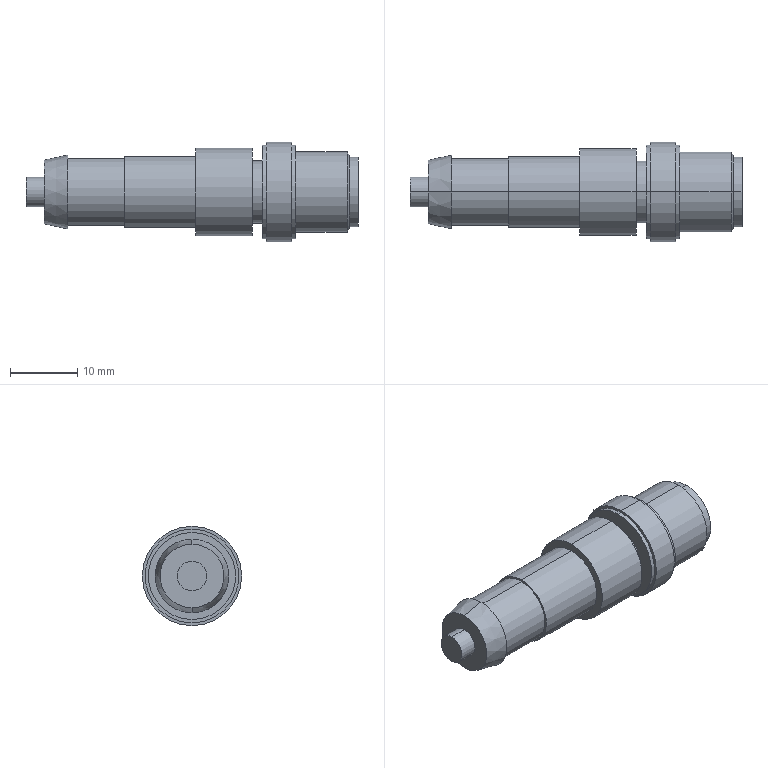Part | STEP file | OP-88071-Part-2-3 | 1 solid | 56 faces | box 49.5 x 14.8 x 14.8 mm | volume 4659 mm3 | cylinder 33 | plane 19 | cone 4 | commonest cylinder face diameters 1 x8 14 x4 8.6 x3 1.2 x2 4.4 x2 9.3 x2
STEP:
#1=CARTESIAN_POINT('',(81.5,2.076,2.924));
#2=VERTEX_POINT('',#1);
#3=CARTESIAN_POINT('',(81.5,2.5,1.9));
#4=VERTEX_POINT('',#3);
#5=CARTESIAN_POINT('',(81.5,2.5,2.5));
#6=DIRECTION('',(1.,0.,0.));
#7=DIRECTION('',(0.,1.,0.));
#8=AXIS2_PLACEMENT_3D('',#5,#6,#7);
#9=CIRCLE('',#8,0.6);
#10=EDGE_CURVE('',#2,#4,#9,.T.);
#11=ORIENTED_EDGE('',*,*,#10,.T.);
#12=CARTESIAN_POINT('',(87.9,2.5,1.9));
#13=VERTEX_POINT('',#12);
#14=CARTESIAN_POINT('',(81.5,2.5,1.9));
#15=DIRECTION('',(1.,0.,0.));
#16=VECTOR('',#15,1000.);
#17=LINE('',#14,#16);
#18=EDGE_CURVE('',#4,#13,#17,.T.);
#19=ORIENTED_EDGE('',*,*,#18,.T.);
#20=CARTESIAN_POINT('',(87.9,2.076,2.924));
#21=VERTEX_POINT('',#20);
#22=CARTESIAN_POINT('',(87.9,2.5,2.5));
#23=DIRECTION('',(1.,0.,0.));
#24=DIRECTION('',(0.,1.,0.));
#25=AXIS2_PLACEMENT_3D('',#22,#23,#24);
#26=CIRCLE('',#25,0.6);
#27=EDGE_CURVE('',#21,#13,#26,.T.);
#28=ORIENTED_EDGE('',*,*,#27,.F.);
#29=CARTESIAN_POINT('',(81.5,2.076,2.924));
#30=DIRECTION('',(1.,0.,0.));
#31=VECTOR('',#30,1000.);
#32=LINE('',#29,#31);
#33=EDGE_CURVE('',#2,#21,#32,.T.);
#34=ORIENTED_EDGE('',*,*,#33,.F.);
#35=EDGE_LOOP('',(#11,#19,#28,#34));
#36=FACE_OUTER_BOUND('',#35,.T.);
#37=CARTESIAN_POINT('',(81.5,2.5,2.5));
#38=DIRECTION('',(1.,0.,0.));
#39=DIRECTION('',(0.,0.,-1.));
#40=AXIS2_PLACEMENT_3D('',#37,#38,#39);
#41=CYLINDRICAL_SURFACE('',#40,0.6);
#42=ADVANCED_FACE('',(#36),#41,.T.);
#43=CARTESIAN_POINT('',(81.5,-2.5,-0.5));
#44=VERTEX_POINT('',#43);
#45=CARTESIAN_POINT('',(81.5,-2.5,0.5));
#46=VERTEX_POINT('',#45);
#47=CARTESIAN_POINT('',(81.5,-2.5,0.));
#48=DIRECTION('',(1.,0.,0.));
#49=DIRECTION('',(0.,1.,0.));
#50=AXIS2_PLACEMENT_3D('',#47,#48,#49);
#51=CIRCLE('',#50,0.5);
#52=EDGE_CURVE('',#44,#46,#51,.T.);
#53=ORIENTED_EDGE('',*,*,#52,.T.);
#54=CARTESIAN_POINT('',(87.9,-2.5,0.5));
#55=VERTEX_POINT('',#54);
#56=CARTESIAN_POINT('',(81.5,-2.5,0.5));
#57=DIRECTION('',(1.,0.,0.));
#58=VECTOR('',#57,1000.);
#59=LINE('',#56,#58);
#60=EDGE_CURVE('',#46,#55,#59,.T.);
#61=ORIENTED_EDGE('',*,*,#60,.T.);
#62=CARTESIAN_POINT('',(87.9,-2.5,-0.5));
#63=VERTEX_POINT('',#62);
#64=CARTESIAN_POINT('',(87.9,-2.5,0.));
#65=DIRECTION('',(1.,0.,0.));
#66=DIRECTION('',(0.,1.,0.));
#67=AXIS2_PLACEMENT_3D('',#64,#65,#66);
#68=CIRCLE('',#67,0.5);
#69=EDGE_CURVE('',#63,#55,#68,.T.);
#70=ORIENTED_EDGE('',*,*,#69,.F.);
#71=CARTESIAN_POINT('',(81.5,-2.5,-0.5));
#72=DIRECTION('',(1.,0.,0.));
#73=VECTOR('',#72,1000.);
#74=LINE('',#71,#73);
#75=EDGE_CURVE('',#44,#63,#74,.T.);
#76=ORIENTED_EDGE('',*,*,#75,.F.);
#77=EDGE_LOOP('',(#53,#61,#70,#76));
#78=FACE_OUTER_BOUND('',#77,.T.);
#79=CARTESIAN_POINT('',(81.5,-2.5,0.));
#80=DIRECTION('',(1.,0.,0.));
#81=DIRECTION('',(0.,0.,-1.));
#82=AXIS2_PLACEMENT_3D('',#79,#80,#81);
#83=CYLINDRICAL_SURFACE('',#82,0.5);
#84=ADVANCED_FACE('',(#78),#83,.T.);
#85=CARTESIAN_POINT('',(81.5,0.,2.));
#86=VERTEX_POINT('',#85);
#87=CARTESIAN_POINT('',(81.5,0.,3.));
#88=VERTEX_POINT('',#87);
#89=CARTESIAN_POINT('',(81.5,0.,2.5));
#90=DIRECTION('',(1.,0.,0.));
#91=DIRECTION('',(0.,1.,0.));
#92=AXIS2_PLACEMENT_3D('',#89,#90,#91);
#93=CIRCLE('',#92,0.5);
#94=EDGE_CURVE('',#86,#88,#93,.T.);
#95=ORIENTED_EDGE('',*,*,#94,.T.);
#96=CARTESIAN_POINT('',(87.9,0.,3.));
#97=VERTEX_POINT('',#96);
#98=CARTESIAN_POINT('',(81.5,0.,3.));
#99=DIRECTION('',(1.,0.,0.));
#100=VECTOR('',#99,1000.);
#101=LINE('',#98,#100);
#102=EDGE_CURVE('',#88,#97,#101,.T.);
#103=ORIENTED_EDGE('',*,*,#102,.T.);
#104=CARTESIAN_POINT('',(87.9,0.,2.));
#105=VERTEX_POINT('',#104);
#106=CARTESIAN_POINT('',(87.9,0.,2.5));
#107=DIRECTION('',(1.,0.,0.));
#108=DIRECTION('',(0.,1.,0.));
#109=AXIS2_PLACEMENT_3D('',#106,#107,#108);
#110=CIRCLE('',#109,0.5);
#111=EDGE_CURVE('',#105,#97,#110,.T.);
#112=ORIENTED_EDGE('',*,*,#111,.F.);
#113=CARTESIAN_POINT('',(81.5,0.,2.));
#114=DIRECTION('',(1.,0.,0.));
#115=VECTOR('',#114,1000.);
#116=LINE('',#113,#115);
#117=EDGE_CURVE('',#86,#105,#116,.T.);
#118=ORIENTED_EDGE('',*,*,#117,.F.);
#119=EDGE_LOOP('',(#95,#103,#112,#118));
#120=FACE_OUTER_BOUND('',#119,.T.);
#121=CARTESIAN_POINT('',(81.5,0.,2.5));
#122=DIRECTION('',(1.,0.,0.));
#123=DIRECTION('',(0.,0.,-1.));
#124=AXIS2_PLACEMENT_3D('',#121,#122,#123);
#125=CYLINDRICAL_SURFACE('',#124,0.5);
#126=ADVANCED_FACE('',(#120),#125,.T.);
#127=CARTESIAN_POINT('',(81.5,0.,-3.));
#128=VERTEX_POINT('',#127);
#129=CARTESIAN_POINT('',(81.5,0.,-2.));
#130=VERTEX_POINT('',#129);
#131=CARTESIAN_POINT('',(81.5,0.,-2.5));
#132=DIRECTION('',(1.,0.,0.));
#133=DIRECTION('',(0.,1.,0.));
#134=AXIS2_PLACEMENT_3D('',#131,#132,#133);
#135=CIRCLE('',#134,0.5);
#136=EDGE_CURVE('',#128,#130,#135,.T.);
#137=ORIENTED_EDGE('',*,*,#136,.T.);
#138=CARTESIAN_POINT('',(87.9,0.,-2.));
#139=VERTEX_POINT('',#138);
#140=CARTESIAN_POINT('',(81.5,0.,-2.));
#141=DIRECTION('',(1.,0.,0.));
#142=VECTOR('',#141,1000.);
#143=LINE('',#140,#142);
#144=EDGE_CURVE('',#130,#139,#143,.T.);
#145=ORIENTED_EDGE('',*,*,#144,.T.);
#146=CARTESIAN_POINT('',(87.9,0.,-3.));
#147=VERTEX_POINT('',#146);
#148=CARTESIAN_POINT('',(87.9,0.,-2.5));
#149=DIRECTION('',(1.,0.,0.));
#150=DIRECTION('',(0.,1.,0.));
#151=AXIS2_PLACEMENT_3D('',#148,#149,#150);
#152=CIRCLE('',#151,0.5);
#153=EDGE_CURVE('',#147,#139,#152,.T.);
#154=ORIENTED_EDGE('',*,*,#153,.F.);
#155=CARTESIAN_POINT('',(81.5,0.,-3.));
#156=DIRECTION('',(1.,0.,0.));
#157=VECTOR('',#156,1000.);
#158=LINE('',#155,#157);
#159=EDGE_CURVE('',#128,#147,#158,.T.);
#160=ORIENTED_EDGE('',*,*,#159,.F.);
#161=EDGE_LOOP('',(#137,#145,#154,#160));
#162=FACE_OUTER_BOUND('',#161,.T.);
#163=CARTESIAN_POINT('',(81.5,0.,-2.5));
#164=DIRECTION('',(1.,0.,0.));
#165=DIRECTION('',(0.,0.,-1.));
#166=AXIS2_PLACEMENT_3D('',#163,#164,#165);
#167=CYLINDRICAL_SURFACE('',#166,0.5);
#168=ADVANCED_FACE('',(#162),#167,.T.);
#169=CARTESIAN_POINT('',(81.5,2.5,-0.5));
#170=VERTEX_POINT('',#169);
#171=CARTESIAN_POINT('',(81.5,2.5,0.5));
#172=VERTEX_POINT('',#171);
#173=CARTESIAN_POINT('',(81.5,2.5,0.));
#174=DIRECTION('',(1.,0.,0.));
#175=DIRECTION('',(0.,1.,0.));
#176=AXIS2_PLACEMENT_3D('',#173,#174,#175);
#177=CIRCLE('',#176,0.5);
#178=EDGE_CURVE('',#170,#172,#177,.T.);
#179=ORIENTED_EDGE('',*,*,#178,.T.);
#180=CARTESIAN_POINT('',(87.9,2.5,0.5));
#181=VERTEX_POINT('',#180);
#182=CARTESIAN_POINT('',(81.5,2.5,0.5));
#183=DIRECTION('',(1.,0.,0.));
#184=VECTOR('',#183,1000.);
#185=LINE('',#182,#184);
#186=EDGE_CURVE('',#172,#181,#185,.T.);
#187=ORIENTED_EDGE('',*,*,#186,.T.);
#188=CARTESIAN_POINT('',(87.9,2.5,-0.5));
#189=VERTEX_POINT('',#188);
#190=CARTESIAN_POINT('',(87.9,2.5,0.));
#191=DIRECTION('',(-1.,0.,0.));
#192=DIRECTION('',(0.,0.,1.));
#193=AXIS2_PLACEMENT_3D('',#190,#191,#192);
#194=CIRCLE('',#193,0.5);
#195=EDGE_CURVE('',#181,#189,#194,.T.);
#196=ORIENTED_EDGE('',*,*,#195,.T.);
#197=CARTESIAN_POINT('',(81.5,2.5,-0.5));
#198=DIRECTION('',(1.,0.,0.));
#199=VECTOR('',#198,1000.);
#200=LINE('',#197,#199);
#201=EDGE_CURVE('',#170,#189,#200,.T.);
#202=ORIENTED_EDGE('',*,*,#201,.F.);
#203=EDGE_LOOP('',(#179,#187,#196,#202));
#204=FACE_OUTER_BOUND('',#203,.T.);
#205=CARTESIAN_POINT('',(81.5,2.5,0.));
#206=DIRECTION('',(1.,0.,0.));
#207=DIRECTION('',(0.,0.,-1.));
#208=AXIS2_PLACEMENT_3D('',#205,#206,#207);
#209=CYLINDRICAL_SURFACE('',#208,0.5);
#210=ADVANCED_FACE('',(#204),#209,.T.);
#211=CARTESIAN_POINT('',(81.5,0.,4.3));
#212=VERTEX_POINT('',#211);
#213=CARTESIAN_POINT('',(81.5,0.,-4.3));
#214=VERTEX_POINT('',#213);
#215=CARTESIAN_POINT('',(81.5,0.,0.));
#216=DIRECTION('',(1.,0.,0.));
#217=DIRECTION('',(0.,1.,0.));
#218=AXIS2_PLACEMENT_3D('',#215,#216,#217);
#219=CIRCLE('',#218,4.3);
#220=EDGE_CURVE('',#212,#214,#219,.T.);
#221=ORIENTED_EDGE('',*,*,#220,.F.);
#222=CARTESIAN_POINT('',(87.9,0.,4.3));
#223=VERTEX_POINT('',#222);
#224=CARTESIAN_POINT('',(81.5,0.,4.3));
#225=DIRECTION('',(1.,0.,0.));
#226=VECTOR('',#225,1000.);
#227=LINE('',#224,#226);
#228=EDGE_CURVE('',#212,#223,#227,.T.);
#229=ORIENTED_EDGE('',*,*,#228,.T.);
#230=CARTESIAN_POINT('',(87.9,0.,-4.3));
#231=VERTEX_POINT('',#230);
#232=CARTESIAN_POINT('',(87.9,0.,0.));
#233=DIRECTION('',(-1.,0.,0.));
#234=DIRECTION('',(0.,0.,1.));
#235=AXIS2_PLACEMENT_3D('',#232,#233,#234);
#236=CIRCLE('',#235,4.3);
#237=EDGE_CURVE('',#231,#223,#236,.T.);
#238=ORIENTED_EDGE('',*,*,#237,.F.);
#239=CARTESIAN_POINT('',(81.5,0.,-4.3));
#240=DIRECTION('',(1.,0.,0.));
#241=VECTOR('',#240,1000.);
#242=LINE('',#239,#241);
#243=EDGE_CURVE('',#214,#231,#242,.T.);
#244=ORIENTED_EDGE('',*,*,#243,.F.);
#245=EDGE_LOOP('',(#221,#229,#238,#244));
#246=FACE_OUTER_BOUND('',#245,.T.);
#247=CARTESIAN_POINT('',(81.5,0.,0.));
#248=DIRECTION('',(1.,0.,0.));
#249=DIRECTION('',(0.,0.,-1.));
#250=AXIS2_PLACEMENT_3D('',#247,#248,#249);
#251=CYLINDRICAL_SURFACE('',#250,4.3);
#252=ADVANCED_FACE('',(#246),#251,.F.);
#253=CARTESIAN_POINT('',(81.5,3.435,2.587));
#254=VERTEX_POINT('',#253);
#255=CARTESIAN_POINT('',(81.5,0.,0.));
#256=DIRECTION('',(1.,0.,0.));
#257=DIRECTION('',(0.,1.,0.));
#258=AXIS2_PLACEMENT_3D('',#255,#256,#257);
#259=CIRCLE('',#258,4.3);
#260=EDGE_CURVE('',#214,#254,#259,.T.);
#261=ORIENTED_EDGE('',*,*,#260,.F.);
#262=ORIENTED_EDGE('',*,*,#243,.T.);
#263=CARTESIAN_POINT('',(87.9,3.435,2.587));
#264=VERTEX_POINT('',#263);
#265=CARTESIAN_POINT('',(87.9,0.,0.));
#266=DIRECTION('',(-1.,0.,0.));
#267=DIRECTION('',(0.,0.,1.));
#268=AXIS2_PLACEMENT_3D('',#265,#266,#267);
#269=CIRCLE('',#268,4.3);
#270=EDGE_CURVE('',#264,#231,#269,.T.);
#271=ORIENTED_EDGE('',*,*,#270,.F.);
#272=CARTESIAN_POINT('',(81.5,3.435,2.587));
#273=DIRECTION('',(1.,0.,0.));
#274=VECTOR('',#273,1000.);
#275=LINE('',#272,#274);
#276=EDGE_CURVE('',#254,#264,#275,.T.);
#277=ORIENTED_EDGE('',*,*,#276,.F.);
#278=EDGE_LOOP('',(#261,#262,#271,#277));
#279=FACE_OUTER_BOUND('',#278,.T.);
#280=CARTESIAN_POINT('',(81.5,0.,0.));
#281=DIRECTION('',(1.,0.,0.));
#282=DIRECTION('',(0.,0.,-1.));
#283=AXIS2_PLACEMENT_3D('',#280,#281,#282);
#284=CYLINDRICAL_SURFACE('',#283,4.3);
#285=ADVANCED_FACE('',(#279),#284,.F.);
#286=CARTESIAN_POINT('',(86.6,0.,-5.2));
#287=VERTEX_POINT('',#286);
#288=CARTESIAN_POINT('',(86.6,0.,5.2));
#289=VERTEX_POINT('',#288);
#290=CARTESIAN_POINT('',(86.6,0.,0.));
#291=DIRECTION('',(1.,0.,0.));
#292=DIRECTION('',(0.,0.,-1.));
#293=AXIS2_PLACEMENT_3D('',#290,#291,#292);
#294=CIRCLE('',#293,5.2);
#295=EDGE_CURVE('',#287,#289,#294,.T.);
#296=ORIENTED_EDGE('',*,*,#295,.T.);
#297=CARTESIAN_POINT('',(87.9,0.,5.2));
#298=VERTEX_POINT('',#297);
#299=CARTESIAN_POINT('',(87.9,0.,5.2));
#300=DIRECTION('',(1.,0.,0.));
#301=VECTOR('',#300,1000.);
#302=LINE('',#299,#301);
#303=EDGE_CURVE('',#289,#298,#302,.T.);
#304=ORIENTED_EDGE('',*,*,#303,.T.);
#305=CARTESIAN_POINT('',(87.9,0.,-5.2));
#306=VERTEX_POINT('',#305);
#307=CARTESIAN_POINT('',(87.9,0.,0.));
#308=DIRECTION('',(1.,0.,0.));
#309=DIRECTION('',(0.,0.,-1.));
#310=AXIS2_PLACEMENT_3D('',#307,#308,#309);
#311=CIRCLE('',#310,5.2);
#312=EDGE_CURVE('',#306,#298,#311,.T.);
#313=ORIENTED_EDGE('',*,*,#312,.F.);
#314=CARTESIAN_POINT('',(87.9,0.,-5.2));
#315=DIRECTION('',(1.,0.,0.));
#316=VECTOR('',#315,1000.);
#317=LINE('',#314,#316);
#318=EDGE_CURVE('',#287,#306,#317,.T.);
#319=ORIENTED_EDGE('',*,*,#318,.F.);
#320=EDGE_LOOP('',(#296,#304,#313,#319));
#321=FACE_OUTER_BOUND('',#320,.T.);
#322=CARTESIAN_POINT('',(87.9,0.,0.));
#323=DIRECTION('',(1.,0.,0.));
#324=DIRECTION('',(0.,0.,-1.));
#325=AXIS2_PLACEMENT_3D('',#322,#323,#324);
#326=CYLINDRICAL_SURFACE('',#325,5.2);
#327=ADVANCED_FACE('',(#321),#326,.T.);
#328=CARTESIAN_POINT('',(86.6,0.,-5.45));
#329=VERTEX_POINT('',#328);
#330=CARTESIAN_POINT('',(86.6,0.,5.45));
#331=VERTEX_POINT('',#330);
#332=CARTESIAN_POINT('',(86.6,0.,0.));
#333=DIRECTION('',(1.,0.,0.));
#334=DIRECTION('',(0.,0.,-1.));
#335=AXIS2_PLACEMENT_3D('',#332,#333,#334);
#336=CIRCLE('',#335,5.45);
#337=EDGE_CURVE('',#329,#331,#336,.T.);
#338=ORIENTED_EDGE('',*,*,#337,.F.);
#339=CARTESIAN_POINT('',(86.3,0.,-6.));
#340=VERTEX_POINT('',#339);
#341=CARTESIAN_POINT('',(86.3,0.,-6.));
#342=DIRECTION('',(-0.4789,0.,-0.8779));
#343=VECTOR('',#342,1000.);
#344=LINE('',#341,#343);
#345=EDGE_CURVE('',#329,#340,#344,.T.);
#346=ORIENTED_EDGE('',*,*,#345,.T.);
#347=CARTESIAN_POINT('',(86.3,0.,6.));
#348=VERTEX_POINT('',#347);
#349=CARTESIAN_POINT('',(86.3,0.,0.));
#350=DIRECTION('',(1.,0.,0.));
#351=DIRECTION('',(0.,0.,-1.));
#352=AXIS2_PLACEMENT_3D('',#349,#350,#351);
#353=CIRCLE('',#352,6.);
#354=EDGE_CURVE('',#340,#348,#353,.T.);
#355=ORIENTED_EDGE('',*,*,#354,.T.);
#356=CARTESIAN_POINT('',(86.3,0.,6.));
#357=DIRECTION('',(-0.4789,0.,0.8779));
#358=VECTOR('',#357,1000.);
#359=LINE('',#356,#358);
#360=EDGE_CURVE('',#331,#348,#359,.T.);
#361=ORIENTED_EDGE('',*,*,#360,.F.);
#362=EDGE_LOOP('',(#338,#346,#355,#361));
#363=FACE_OUTER_BOUND('',#362,.T.);
#364=CARTESIAN_POINT('',(86.3,0.,0.));
#365=DIRECTION('',(-1.,0.,0.));
#366=DIRECTION('',(0.,0.,1.));
#367=AXIS2_PLACEMENT_3D('',#364,#365,#366);
#368=CONICAL_SURFACE('',#367,6.,1.071);
#369=ADVANCED_FACE('',(#363),#368,.T.);
#370=CARTESIAN_POINT('',(78.6,0.,-6.));
#371=VERTEX_POINT('',#370);
#372=CARTESIAN_POINT('',(78.6,0.,6.));
#373=VERTEX_POINT('',#372);
#374=CARTESIAN_POINT('',(78.6,0.,0.));
#375=DIRECTION('',(1.,0.,0.));
#376=DIRECTION('',(0.,0.,-1.));
#377=AXIS2_PLACEMENT_3D('',#374,#375,#376);
#378=CIRCLE('',#377,6.);
#379=EDGE_CURVE('',#371,#373,#378,.T.);
#380=ORIENTED_EDGE('',*,*,#379,.T.);
#381=CARTESIAN_POINT('',(87.9,0.,6.));
#382=DIRECTION('',(1.,0.,0.));
#383=VECTOR('',#382,1000.);
#384=LINE('',#381,#383);
#385=EDGE_CURVE('',#373,#348,#384,.T.);
#386=ORIENTED_EDGE('',*,*,#385,.T.);
#387=ORIENTED_EDGE('',*,*,#354,.F.);
#388=CARTESIAN_POINT('',(87.9,0.,-6.));
#389=DIRECTION('',(1.,0.,0.));
#390=VECTOR('',#389,1000.);
#391=LINE('',#388,#390);
#392=EDGE_CURVE('',#371,#340,#391,.T.);
#393=ORIENTED_EDGE('',*,*,#392,.F.);
#394=EDGE_LOOP('',(#380,#386,#387,#393));
#395=FACE_OUTER_BOUND('',#394,.T.);
#396=CARTESIAN_POINT('',(87.9,0.,0.));
#397=DIRECTION('',(1.,0.,0.));
#398=DIRECTION('',(0.,0.,-1.));
#399=AXIS2_PLACEMENT_3D('',#396,#397,#398);
#400=CYLINDRICAL_SURFACE('',#399,6.);
#401=ADVANCED_FACE('',(#395),#400,.T.);
#402=CARTESIAN_POINT('',(78.,0.,-7.));
#403=VERTEX_POINT('',#402);
#404=CARTESIAN_POINT('',(78.,0.,7.));
#405=VERTEX_POINT('',#404);
#406=CARTESIAN_POINT('',(78.,0.,0.));
#407=DIRECTION('',(1.,0.,0.));
#408=DIRECTION('',(0.,0.,-1.));
#409=AXIS2_PLACEMENT_3D('',#406,#407,#408);
#410=CIRCLE('',#409,7.);
#411=EDGE_CURVE('',#403,#405,#410,.T.);
#412=ORIENTED_EDGE('',*,*,#411,.T.);
#413=CARTESIAN_POINT('',(78.6,0.,7.));
#414=VERTEX_POINT('',#413);
#415=CARTESIAN_POINT('',(87.9,0.,7.));
#416=DIRECTION('',(1.,0.,0.));
#417=VECTOR('',#416,1000.);
#418=LINE('',#415,#417);
#419=EDGE_CURVE('',#405,#414,#418,.T.);
#420=ORIENTED_EDGE('',*,*,#419,.T.);
#421=CARTESIAN_POINT('',(78.6,0.,-7.));
#422=VERTEX_POINT('',#421);
#423=CARTESIAN_POINT('',(78.6,0.,0.));
#424=DIRECTION('',(1.,0.,0.));
#425=DIRECTION('',(0.,0.,-1.));
#426=AXIS2_PLACEMENT_3D('',#423,#424,#425);
#427=CIRCLE('',#426,7.);
#428=EDGE_CURVE('',#422,#414,#427,.T.);
#429=ORIENTED_EDGE('',*,*,#428,.F.);
#430=CARTESIAN_POINT('',(87.9,0.,-7.));
#431=DIRECTION('',(1.,0.,0.));
#432=VECTOR('',#431,1000.);
#433=LINE('',#430,#432);
#434=EDGE_CURVE('',#403,#422,#433,.T.);
#435=ORIENTED_EDGE('',*,*,#434,.F.);
#436=EDGE_LOOP('',(#412,#420,#429,#435));
#437=FACE_OUTER_BOUND('',#436,.T.);
#438=CARTESIAN_POINT('',(87.9,0.,0.));
#439=DIRECTION('',(1.,0.,0.));
#440=DIRECTION('',(0.,0.,-1.));
#441=AXIS2_PLACEMENT_3D('',#438,#439,#440);
#442=CYLINDRICAL_SURFACE('',#441,7.);
#443=ADVANCED_FACE('',(#437),#442,.T.);
#444=CARTESIAN_POINT('',(74.2,0.,-7.4));
#445=VERTEX_POINT('',#444);
#446=CARTESIAN_POINT('',(74.2,0.,7.4));
#447=VERTEX_POINT('',#446);
#448=CARTESIAN_POINT('',(74.2,0.,0.));
#449=DIRECTION('',(1.,0.,0.));
#450=DIRECTION('',(0.,0.,-1.));
#451=AXIS2_PLACEMENT_3D('',#448,#449,#450);
#452=CIRCLE('',#451,7.4);
#453=EDGE_CURVE('',#445,#447,#452,.T.);
#454=ORIENTED_EDGE('',*,*,#453,.T.);
#455=CARTESIAN_POINT('',(78.,0.,7.4));
#456=VERTEX_POINT('',#455);
#457=CARTESIAN_POINT('',(87.9,0.,7.4));
#458=DIRECTION('',(1.,0.,0.));
#459=VECTOR('',#458,1000.);
#460=LINE('',#457,#459);
#461=EDGE_CURVE('',#447,#456,#460,.T.);
#462=ORIENTED_EDGE('',*,*,#461,.T.);
#463=CARTESIAN_POINT('',(78.,0.,-7.4));
#464=VERTEX_POINT('',#463);
#465=CARTESIAN_POINT('',(78.,0.,0.));
#466=DIRECTION('',(1.,0.,0.));
#467=DIRECTION('',(0.,0.,-1.));
#468=AXIS2_PLACEMENT_3D('',#465,#466,#467);
#469=CIRCLE('',#468,7.4);
#470=EDGE_CURVE('',#464,#456,#469,.T.);
#471=ORIENTED_EDGE('',*,*,#470,.F.);
#472=CARTESIAN_POINT('',(87.9,0.,-7.4));
#473=DIRECTION('',(1.,0.,0.));
#474=VECTOR('',#473,1000.);
#475=LINE('',#472,#474);
#476=EDGE_CURVE('',#445,#464,#475,.T.);
#477=ORIENTED_EDGE('',*,*,#476,.F.);
#478=EDGE_LOOP('',(#454,#462,#471,#477));
#479=FACE_OUTER_BOUND('',#478,.T.);
#480=CARTESIAN_POINT('',(87.9,0.,0.));
#481=DIRECTION('',(1.,0.,0.));
#482=DIRECTION('',(0.,0.,-1.));
#483=AXIS2_PLACEMENT_3D('',#480,#481,#482);
#484=CYLINDRICAL_SURFACE('',#483,7.4);
#485=ADVANCED_FACE('',(#479),#484,.T.);
#486=CARTESIAN_POINT('',(73.6,0.,-7.));
#487=VERTEX_POINT('',#486);
#488=CARTESIAN_POINT('',(73.6,0.,7.));
#489=VERTEX_POINT('',#488);
#490=CARTESIAN_POINT('',(73.6,0.,0.));
#491=DIRECTION('',(1.,0.,0.));
#492=DIRECTION('',(0.,0.,-1.));
#493=AXIS2_PLACEMENT_3D('',#490,#491,#492);
#494=CIRCLE('',#493,7.);
#495=EDGE_CURVE('',#487,#489,#494,.T.);
#496=ORIENTED_EDGE('',*,*,#495,.T.);
#497=CARTESIAN_POINT('',(74.2,0.,7.));
#498=VERTEX_POINT('',#497);
#499=CARTESIAN_POINT('',(87.9,0.,7.));
#500=DIRECTION('',(1.,0.,0.));
#501=VECTOR('',#500,1000.);
#502=LINE('',#499,#501);
#503=EDGE_CURVE('',#489,#498,#502,.T.);
#504=ORIENTED_EDGE('',*,*,#503,.T.);
#505=CARTESIAN_POINT('',(74.2,0.,-7.));
#506=VERTEX_POINT('',#505);
#507=CARTESIAN_POINT('',(74.2,0.,0.));
#508=DIRECTION('',(1.,0.,0.));
#509=DIRECTION('',(0.,0.,-1.));
#510=AXIS2_PLACEMENT_3D('',#507,#508,#509);
#511=CIRCLE('',#510,7.);
#512=EDGE_CURVE('',#506,#498,#511,.T.);
#513=ORIENTED_EDGE('',*,*,#512,.F.);
#514=CARTESIAN_POINT('',(87.9,0.,-7.));
#515=DIRECTION('',(1.,0.,0.));
#516=VECTOR('',#515,1000.);
#517=LINE('',#514,#516);
#518=EDGE_CURVE('',#487,#506,#517,.T.);
#519=ORIENTED_EDGE('',*,*,#518,.F.);
#520=EDGE_LOOP('',(#496,#504,#513,#519));
#521=FACE_OUTER_BOUND('',#520,.T.);
#522=CARTESIAN_POINT('',(87.9,0.,0.));
#523=DIRECTION('',(1.,0.,0.));
#524=DIRECTION('',(0.,0.,-1.));
#525=AXIS2_PLACEMENT_3D('',#522,#523,#524);
#526=CYLINDRICAL_SURFACE('',#525,7.);
#527=ADVANCED_FACE('',(#521),#526,.T.);
#528=CARTESIAN_POINT('',(72.1,0.,-4.65));
#529=VERTEX_POINT('',#528);
#530=CARTESIAN_POINT('',(72.1,0.,4.65));
#531=VERTEX_POINT('',#530);
#532=CARTESIAN_POINT('',(72.1,0.,0.));
#533=DIRECTION('',(1.,0.,0.));
#534=DIRECTION('',(0.,0.,-1.));
#535=AXIS2_PLACEMENT_3D('',#532,#533,#534);
#536=CIRCLE('',#535,4.65);
#537=EDGE_CURVE('',#529,#531,#536,.T.);
#538=ORIENTED_EDGE('',*,*,#537,.T.);
#539=CARTESIAN_POINT('',(73.6,0.,4.65));
#540=VERTEX_POINT('',#539);
#541=CARTESIAN_POINT('',(87.9,0.,4.65));
#542=DIRECTION('',(1.,0.,0.));
#543=VECTOR('',#542,1000.);
#544=LINE('',#541,#543);
#545=EDGE_CURVE('',#531,#540,#544,.T.);
#546=ORIENTED_EDGE('',*,*,#545,.T.);
#547=CARTESIAN_POINT('',(73.6,0.,-4.65));
#548=VERTEX_POINT('',#547);
#549=CARTESIAN_POINT('',(73.6,0.,0.));
#550=DIRECTION('',(1.,0.,0.));
#551=DIRECTION('',(0.,0.,-1.));
#552=AXIS2_PLACEMENT_3D('',#549,#550,#551);
#553=CIRCLE('',#552,4.65);
#554=EDGE_CURVE('',#548,#540,#553,.T.);
#555=ORIENTED_EDGE('',*,*,#554,.F.);
#556=CARTESIAN_POINT('',(87.9,0.,-4.65));
#557=DIRECTION('',(1.,0.,0.));
#558=VECTOR('',#557,1000.);
#559=LINE('',#556,#558);
#560=EDGE_CURVE('',#529,#548,#559,.T.);
#561=ORIENTED_EDGE('',*,*,#560,.F.);
#562=EDGE_LOOP('',(#538,#546,#555,#561));
#563=FACE_OUTER_BOUND('',#562,.T.);
#564=CARTESIAN_POINT('',(87.9,0.,0.));
#565=DIRECTION('',(1.,0.,0.));
#566=DIRECTION('',(0.,0.,-1.));
#567=AXIS2_PLACEMENT_3D('',#564,#565,#566);
#568=CYLINDRICAL_SURFACE('',#567,4.65);
#569=ADVANCED_FACE('',(#563),#568,.T.);
#570=CARTESIAN_POINT('',(63.7,0.,-6.5));
#571=VERTEX_POINT('',#570);
#572=CARTESIAN_POINT('',(63.7,0.,6.5));
#573=VERTEX_POINT('',#572);
#574=CARTESIAN_POINT('',(63.7,0.,0.));
#575=DIRECTION('',(1.,0.,0.));
#576=DIRECTION('',(0.,0.,-1.));
#577=AXIS2_PLACEMENT_3D('',#574,#575,#576);
#578=CIRCLE('',#577,6.5);
#579=EDGE_CURVE('',#571,#573,#578,.T.);
#580=ORIENTED_EDGE('',*,*,#579,.T.);
#581=CARTESIAN_POINT('',(72.1,0.,6.5));
#582=VERTEX_POINT('',#581);
#583=CARTESIAN_POINT('',(87.9,0.,6.5));
#584=DIRECTION('',(1.,0.,0.));
#585=VECTOR('',#584,1000.);
#586=LINE('',#583,#585);
#587=EDGE_CURVE('',#573,#582,#586,.T.);
#588=ORIENTED_EDGE('',*,*,#587,.T.);
#589=CARTESIAN_POINT('',(72.1,0.,-6.5));
#590=VERTEX_POINT('',#589);
#591=CARTESIAN_POINT('',(72.1,0.,0.));
#592=DIRECTION('',(1.,0.,0.));
#593=DIRECTION('',(0.,0.,-1.));
#594=AXIS2_PLACEMENT_3D('',#591,#592,#593);
#595=CIRCLE('',#594,6.5);
#596=EDGE_CURVE('',#590,#582,#595,.T.);
#597=ORIENTED_EDGE('',*,*,#596,.F.);
#598=CARTESIAN_POINT('',(87.9,0.,-6.5));
#599=DIRECTION('',(1.,0.,0.));
#600=VECTOR('',#599,1000.);
#601=LINE('',#598,#600);
#602=EDGE_CURVE('',#571,#590,#601,.T.);
#603=ORIENTED_EDGE('',*,*,#602,.F.);
#604=EDGE_LOOP('',(#580,#588,#597,#603));
#605=FACE_OUTER_BOUND('',#604,.T.);
#606=CARTESIAN_POINT('',(87.9,0.,0.));
#607=DIRECTION('',(1.,0.,0.));
#608=DIRECTION('',(0.,0.,-1.));
#609=AXIS2_PLACEMENT_3D('',#606,#607,#608);
#610=CYLINDRICAL_SURFACE('',#609,6.5);
#611=ADVANCED_FACE('',(#605),#610,.T.);
#612=CARTESIAN_POINT('',(53.1,0.,-5.3));
#613=VERTEX_POINT('',#612);
#614=CARTESIAN_POINT('',(53.1,0.,5.3));
#615=VERTEX_POINT('',#614);
#616=CARTESIAN_POINT('',(53.1,0.,0.));
#617=DIRECTION('',(1.,0.,0.));
#618=DIRECTION('',(0.,0.,-1.));
#619=AXIS2_PLACEMENT_3D('',#616,#617,#618);
#620=CIRCLE('',#619,5.3);
#621=EDGE_CURVE('',#613,#615,#620,.T.);
#622=ORIENTED_EDGE('',*,*,#621,.T.);
#623=CARTESIAN_POINT('',(63.7,0.,5.3));
#624=VERTEX_POINT('',#623);
#625=CARTESIAN_POINT('',(87.9,0.,5.3));
#626=DIRECTION('',(1.,0.,0.));
#627=VECTOR('',#626,1000.);
#628=LINE('',#625,#627);
#629=EDGE_CURVE('',#615,#624,#628,.T.);
#630=ORIENTED_EDGE('',*,*,#629,.T.);
#631=CARTESIAN_POINT('',(63.7,0.,-5.3));
#632=VERTEX_POINT('',#631);
#633=CARTESIAN_POINT('',(63.7,0.,0.));
#634=DIRECTION('',(1.,0.,0.));
#635=DIRECTION('',(0.,0.,-1.));
#636=AXIS2_PLACEMENT_3D('',#633,#634,#635);
#637=CIRCLE('',#636,5.3);
#638=EDGE_CURVE('',#632,#624,#637,.T.);
#639=ORIENTED_EDGE('',*,*,#638,.F.);
#640=CARTESIAN_POINT('',(87.9,0.,-5.3));
#641=DIRECTION('',(1.,0.,0.));
#642=VECTOR('',#641,1000.);
#643=LINE('',#640,#642);
#644=EDGE_CURVE('',#613,#632,#643,.T.);
#645=ORIENTED_EDGE('',*,*,#644,.F.);
#646=EDGE_LOOP('',(#622,#630,#639,#645));
#647=FACE_OUTER_BOUND('',#646,.T.);
#648=CARTESIAN_POINT('',(87.9,0.,0.));
#649=DIRECTION('',(1.,0.,0.));
#650=DIRECTION('',(0.,0.,-1.));
#651=AXIS2_PLACEMENT_3D('',#648,#649,#650);
#652=CYLINDRICAL_SURFACE('',#651,5.3);
#653=ADVANCED_FACE('',(#647),#652,.T.);
#654=CARTESIAN_POINT('',(44.6,0.,-5.));
#655=VERTEX_POINT('',#654);
#656=CARTESIAN_POINT('',(44.6,0.,5.));
#657=VERTEX_POINT('',#656);
#658=CARTESIAN_POINT('',(44.6,0.,0.));
#659=DIRECTION('',(1.,0.,0.));
#660=DIRECTION('',(0.,0.,-1.));
#661=AXIS2_PLACEMENT_3D('',#658,#659,#660);
#662=CIRCLE('',#661,5.);
#663=EDGE_CURVE('',#655,#657,#662,.T.);
#664=ORIENTED_EDGE('',*,*,#663,.T.);
#665=CARTESIAN_POINT('',(53.1,0.,5.));
#666=VERTEX_POINT('',#665);
#667=CARTESIAN_POINT('',(87.9,0.,5.));
#668=DIRECTION('',(1.,0.,0.));
#669=VECTOR('',#668,1000.);
#670=LINE('',#667,#669);
#671=EDGE_CURVE('',#657,#666,#670,.T.);
#672=ORIENTED_EDGE('',*,*,#671,.T.);
#673=CARTESIAN_POINT('',(53.1,0.,-5.));
#674=VERTEX_POINT('',#673);
#675=CARTESIAN_POINT('',(53.1,0.,0.));
#676=DIRECTION('',(1.,0.,0.));
#677=DIRECTION('',(0.,0.,-1.));
#678=AXIS2_PLACEMENT_3D('',#675,#676,#677);
#679=CIRCLE('',#678,5.);
#680=EDGE_CURVE('',#674,#666,#679,.T.);
#681=ORIENTED_EDGE('',*,*,#680,.F.);
#682=CARTESIAN_POINT('',(87.9,0.,-5.));
#683=DIRECTION('',(1.,0.,0.));
#684=VECTOR('',#683,1000.);
#685=LINE('',#682,#684);
#686=EDGE_CURVE('',#655,#674,#685,.T.);
#687=ORIENTED_EDGE('',*,*,#686,.F.);
#688=EDGE_LOOP('',(#664,#672,#681,#687));
#689=FACE_OUTER_BOUND('',#688,.T.);
#690=CARTESIAN_POINT('',(87.9,0.,0.));
#691=DIRECTION('',(1.,0.,0.));
#692=DIRECTION('',(0.,0.,-1.));
#693=AXIS2_PLACEMENT_3D('',#690,#691,#692);
#694=CYLINDRICAL_SURFACE('',#693,5.);
#695=ADVANCED_FACE('',(#689),#694,.T.);
#696=CARTESIAN_POINT('',(41.1,0.,-4.75));
#697=VERTEX_POINT('',#696);
#698=CARTESIAN_POINT('',(41.1,0.,4.75));
#699=VERTEX_POINT('',#698);
#700=CARTESIAN_POINT('',(41.1,0.,0.));
#701=DIRECTION('',(1.,0.,0.));
#702=DIRECTION('',(0.,0.,-1.));
#703=AXIS2_PLACEMENT_3D('',#700,#701,#702);
#704=CIRCLE('',#703,4.75);
#705=EDGE_CURVE('',#697,#699,#704,.T.);
#706=ORIENTED_EDGE('',*,*,#705,.T.);
#707=CARTESIAN_POINT('',(44.6,0.,5.5));
#708=VERTEX_POINT('',#707);
#709=CARTESIAN_POINT('',(41.1,0.,4.75));
#710=DIRECTION('',(0.9778,0.,0.2095));
#711=VECTOR('',#710,1000.);
#712=LINE('',#709,#711);
#713=EDGE_CURVE('',#699,#708,#712,.T.);
#714=ORIENTED_EDGE('',*,*,#713,.T.);
#715=CARTESIAN_POINT('',(44.6,0.,-5.5));
#716=VERTEX_POINT('',#715);
#717=CARTESIAN_POINT('',(44.6,0.,0.));
#718=DIRECTION('',(1.,0.,0.));
#719=DIRECTION('',(0.,0.,-1.));
#720=AXIS2_PLACEMENT_3D('',#717,#718,#719);
#721=CIRCLE('',#720,5.5);
#722=EDGE_CURVE('',#716,#708,#721,.T.);
#723=ORIENTED_EDGE('',*,*,#722,.F.);
#724=CARTESIAN_POINT('',(41.1,0.,-4.75));
#725=DIRECTION('',(0.9778,0.,-0.2095));
#726=VECTOR('',#725,1000.);
#727=LINE('',#724,#726);
#728=EDGE_CURVE('',#697,#716,#727,.T.);
#729=ORIENTED_EDGE('',*,*,#728,.F.);
#730=EDGE_LOOP('',(#706,#714,#723,#729));
#731=FACE_OUTER_BOUND('',#730,.T.);
#732=CARTESIAN_POINT('',(41.1,0.,0.));
#733=DIRECTION('',(1.,0.,0.));
#734=DIRECTION('',(0.,0.,-1.));
#735=AXIS2_PLACEMENT_3D('',#732,#733,#734);
#736=CONICAL_SURFACE('',#735,4.75,0.2111);
#737=ADVANCED_FACE('',(#731),#736,.T.);
#738=CARTESIAN_POINT('',(38.4,0.,-2.2));
#739=VERTEX_POINT('',#738);
#740=CARTESIAN_POINT('',(38.4,0.,2.2));
#741=VERTEX_POINT('',#740);
#742=CARTESIAN_POINT('',(38.4,0.,0.));
#743=DIRECTION('',(1.,0.,0.));
#744=DIRECTION('',(0.,0.,-1.));
#745=AXIS2_PLACEMENT_3D('',#742,#743,#744);
#746=CIRCLE('',#745,2.2);
#747=EDGE_CURVE('',#739,#741,#746,.T.);
#748=ORIENTED_EDGE('',*,*,#747,.T.);
#749=CARTESIAN_POINT('',(41.1,0.,2.2));
#750=VERTEX_POINT('',#749);
#751=CARTESIAN_POINT('',(87.9,0.,2.2));
#752=DIRECTION('',(1.,0.,0.));
#753=VECTOR('',#752,1000.);
#754=LINE('',#751,#753);
#755=EDGE_CURVE('',#741,#750,#754,.T.);
#756=ORIENTED_EDGE('',*,*,#755,.T.);
#757=CARTESIAN_POINT('',(41.1,0.,-2.2));
#758=VERTEX_POINT('',#757);
#759=CARTESIAN_POINT('',(41.1,0.,0.));
#760=DIRECTION('',(1.,0.,0.));
#761=DIRECTION('',(0.,0.,-1.));
#762=AXIS2_PLACEMENT_3D('',#759,#760,#761);
#763=CIRCLE('',#762,2.2);
#764=EDGE_CURVE('',#758,#750,#763,.T.);
#765=ORIENTED_EDGE('',*,*,#764,.F.);
#766=CARTESIAN_POINT('',(87.9,0.,-2.2));
#767=DIRECTION('',(1.,0.,0.));
#768=VECTOR('',#767,1000.);
#769=LINE('',#766,#768);
#770=EDGE_CURVE('',#739,#758,#769,.T.);
#771=ORIENTED_EDGE('',*,*,#770,.F.);
#772=EDGE_LOOP('',(#748,#756,#765,#771));
#773=FACE_OUTER_BOUND('',#772,.T.);
#774=CARTESIAN_POINT('',(87.9,0.,0.));
#775=DIRECTION('',(1.,0.,0.));
#776=DIRECTION('',(0.,0.,-1.));
#777=AXIS2_PLACEMENT_3D('',#774,#775,#776);
#778=CYLINDRICAL_SURFACE('',#777,2.2);
#779=ADVANCED_FACE('',(#773),#778,.T.);
#780=ORIENTED_EDGE('',*,*,#747,.F.);
#781=CARTESIAN_POINT('',(38.4,0.,0.));
#782=DIRECTION('',(1.,0.,0.));
#783=DIRECTION('',(0.,0.,-1.));
#784=AXIS2_PLACEMENT_3D('',#781,#782,#783);
#785=CIRCLE('',#784,2.2);
#786=EDGE_CURVE('',#741,#739,#785,.T.);
#787=ORIENTED_EDGE('',*,*,#786,.F.);
#788=EDGE_LOOP('',(#780,#787));
#789=FACE_OUTER_BOUND('',#788,.T.);
#790=CARTESIAN_POINT('',(38.4,0.,0.));
#791=DIRECTION('',(1.,0.,0.));
#792=DIRECTION('',(0.,0.,-1.));
#793=AXIS2_PLACEMENT_3D('',#790,#791,#792);
#794=PLANE('',#793);
#795=ADVANCED_FACE('',(#789),#794,.F.);
#796=ORIENTED_EDGE('',*,*,#755,.F.);
#797=ORIENTED_EDGE('',*,*,#786,.T.);
#798=ORIENTED_EDGE('',*,*,#770,.T.);
#799=CARTESIAN_POINT('',(41.1,0.,0.));
#800=DIRECTION('',(1.,0.,0.));
#801=DIRECTION('',(0.,0.,-1.));
#802=AXIS2_PLACEMENT_3D('',#799,#800,#801);
#803=CIRCLE('',#802,2.2);
#804=EDGE_CURVE('',#750,#758,#803,.T.);
#805=ORIENTED_EDGE('',*,*,#804,.F.);
#806=EDGE_LOOP('',(#796,#797,#798,#805));
#807=FACE_OUTER_BOUND('',#806,.T.);
#808=CARTESIAN_POINT('',(87.9,0.,0.));
#809=DIRECTION('',(1.,0.,0.));
#810=DIRECTION('',(0.,0.,-1.));
#811=AXIS2_PLACEMENT_3D('',#808,#809,#810);
#812=CYLINDRICAL_SURFACE('',#811,2.2);
#813=ADVANCED_FACE('',(#807),#812,.T.);
#814=ORIENTED_EDGE('',*,*,#705,.F.);
#815=CARTESIAN_POINT('',(41.1,0.,0.));
#816=DIRECTION('',(1.,0.,0.));
#817=DIRECTION('',(0.,0.,-1.));
#818=AXIS2_PLACEMENT_3D('',#815,#816,#817);
#819=CIRCLE('',#818,4.75);
#820=EDGE_CURVE('',#699,#697,#819,.T.);
#821=ORIENTED_EDGE('',*,*,#820,.F.);
#822=EDGE_LOOP('',(#814,#821));
#823=FACE_OUTER_BOUND('',#822,.T.);
#824=ORIENTED_EDGE('',*,*,#764,.T.);
#825=ORIENTED_EDGE('',*,*,#804,.T.);
#826=EDGE_LOOP('',(#824,#825));
#827=FACE_BOUND('',#826,.T.);
#828=CARTESIAN_POINT('',(41.1,2.2,0.));
#829=DIRECTION('',(1.,0.,0.));
#830=DIRECTION('',(0.,0.,-1.));
#831=AXIS2_PLACEMENT_3D('',#828,#829,#830);
#832=PLANE('',#831);
#833=ADVANCED_FACE('',(#823,#827),#832,.F.);
#834=ORIENTED_EDGE('',*,*,#713,.F.);
#835=ORIENTED_EDGE('',*,*,#820,.T.);
#836=ORIENTED_EDGE('',*,*,#728,.T.);
#837=CARTESIAN_POINT('',(44.6,0.,0.));
#838=DIRECTION('',(1.,0.,0.));
#839=DIRECTION('',(0.,0.,-1.));
#840=AXIS2_PLACEMENT_3D('',#837,#838,#839);
#841=CIRCLE('',#840,5.5);
#842=EDGE_CURVE('',#708,#716,#841,.T.);
#843=ORIENTED_EDGE('',*,*,#842,.F.);
#844=EDGE_LOOP('',(#834,#835,#836,#843));
#845=FACE_OUTER_BOUND('',#844,.T.);
#846=CARTESIAN_POINT('',(41.1,0.,0.));
#847=DIRECTION('',(1.,0.,0.));
#848=DIRECTION('',(0.,0.,-1.));
#849=AXIS2_PLACEMENT_3D('',#846,#847,#848);
#850=CONICAL_SURFACE('',#849,4.75,0.2111);
#851=ADVANCED_FACE('',(#845),#850,.T.);
#852=ORIENTED_EDGE('',*,*,#663,.F.);
#853=CARTESIAN_POINT('',(44.6,0.,0.));
#854=DIRECTION('',(1.,0.,0.));
#855=DIRECTION('',(0.,0.,-1.));
#856=AXIS2_PLACEMENT_3D('',#853,#854,#855);
#857=CIRCLE('',#856,5.);
#858=EDGE_CURVE('',#657,#655,#857,.T.);
#859=ORIENTED_EDGE('',*,*,#858,.F.);
#860=EDGE_LOOP('',(#852,#859));
#861=FACE_BOUND('',#860,.T.);
#862=ORIENTED_EDGE('',*,*,#722,.T.);
#863=ORIENTED_EDGE('',*,*,#842,.T.);
#864=EDGE_LOOP('',(#862,#863));
#865=FACE_OUTER_BOUND('',#864,.T.);
#866=CARTESIAN_POINT('',(44.6,5.5,0.));
#867=DIRECTION('',(-1.,0.,0.));
#868=DIRECTION('',(0.,0.,1.));
#869=AXIS2_PLACEMENT_3D('',#866,#867,#868);
#870=PLANE('',#869);
#871=ADVANCED_FACE('',(#861,#865),#870,.F.);
#872=ORIENTED_EDGE('',*,*,#671,.F.);
#873=ORIENTED_EDGE('',*,*,#858,.T.);
#874=ORIENTED_EDGE('',*,*,#686,.T.);
#875=CARTESIAN_POINT('',(53.1,0.,0.));
#876=DIRECTION('',(1.,0.,0.));
#877=DIRECTION('',(0.,0.,-1.));
#878=AXIS2_PLACEMENT_3D('',#875,#876,#877);
#879=CIRCLE('',#878,5.);
#880=EDGE_CURVE('',#666,#674,#879,.T.);
#881=ORIENTED_EDGE('',*,*,#880,.F.);
#882=EDGE_LOOP('',(#872,#873,#874,#881));
#883=FACE_OUTER_BOUND('',#882,.T.);
#884=CARTESIAN_POINT('',(87.9,0.,0.));
#885=DIRECTION('',(1.,0.,0.));
#886=DIRECTION('',(0.,0.,-1.));
#887=AXIS2_PLACEMENT_3D('',#884,#885,#886);
#888=CYLINDRICAL_SURFACE('',#887,5.);
#889=ADVANCED_FACE('',(#883),#888,.T.);
#890=ORIENTED_EDGE('',*,*,#621,.F.);
#891=CARTESIAN_POINT('',(53.1,0.,0.));
#892=DIRECTION('',(1.,0.,0.));
#893=DIRECTION('',(0.,0.,-1.));
#894=AXIS2_PLACEMENT_3D('',#891,#892,#893);
#895=CIRCLE('',#894,5.3);
#896=EDGE_CURVE('',#615,#613,#895,.T.);
#897=ORIENTED_EDGE('',*,*,#896,.F.);
#898=EDGE_LOOP('',(#890,#897));
#899=FACE_OUTER_BOUND('',#898,.T.);
#900=ORIENTED_EDGE('',*,*,#680,.T.);
#901=ORIENTED_EDGE('',*,*,#880,.T.);
#902=EDGE_LOOP('',(#900,#901));
#903=FACE_BOUND('',#902,.T.);
#904=CARTESIAN_POINT('',(53.1,5.,0.));
#905=DIRECTION('',(1.,0.,0.));
#906=DIRECTION('',(0.,0.,-1.));
#907=AXIS2_PLACEMENT_3D('',#904,#905,#906);
#908=PLANE('',#907);
#909=ADVANCED_FACE('',(#899,#903),#908,.F.);
#910=ORIENTED_EDGE('',*,*,#629,.F.);
#911=ORIENTED_EDGE('',*,*,#896,.T.);
#912=ORIENTED_EDGE('',*,*,#644,.T.);
#913=CARTESIAN_POINT('',(63.7,0.,0.));
#914=DIRECTION('',(1.,0.,0.));
#915=DIRECTION('',(0.,0.,-1.));
#916=AXIS2_PLACEMENT_3D('',#913,#914,#915);
#917=CIRCLE('',#916,5.3);
#918=EDGE_CURVE('',#624,#632,#917,.T.);
#919=ORIENTED_EDGE('',*,*,#918,.F.);
#920=EDGE_LOOP('',(#910,#911,#912,#919));
#921=FACE_OUTER_BOUND('',#920,.T.);
#922=CARTESIAN_POINT('',(87.9,0.,0.));
#923=DIRECTION('',(1.,0.,0.));
#924=DIRECTION('',(0.,0.,-1.));
#925=AXIS2_PLACEMENT_3D('',#922,#923,#924);
#926=CYLINDRICAL_SURFACE('',#925,5.3);
#927=ADVANCED_FACE('',(#921),#926,.T.);
#928=ORIENTED_EDGE('',*,*,#579,.F.);
#929=CARTESIAN_POINT('',(63.7,0.,0.));
#930=DIRECTION('',(1.,0.,0.));
#931=DIRECTION('',(0.,0.,-1.));
#932=AXIS2_PLACEMENT_3D('',#929,#930,#931);
#933=CIRCLE('',#932,6.5);
#934=EDGE_CURVE('',#573,#571,#933,.T.);
#935=ORIENTED_EDGE('',*,*,#934,.F.);
#936=EDGE_LOOP('',(#928,#935));
#937=FACE_OUTER_BOUND('',#936,.T.);
#938=ORIENTED_EDGE('',*,*,#638,.T.);
#939=ORIENTED_EDGE('',*,*,#918,.T.);
#940=EDGE_LOOP('',(#938,#939));
#941=FACE_BOUND('',#940,.T.);
#942=CARTESIAN_POINT('',(63.7,5.3,0.));
#943=DIRECTION('',(1.,0.,0.));
#944=DIRECTION('',(0.,0.,-1.));
#945=AXIS2_PLACEMENT_3D('',#942,#943,#944);
#946=PLANE('',#945);
#947=ADVANCED_FACE('',(#937,#941),#946,.F.);
#948=ORIENTED_EDGE('',*,*,#587,.F.);
#949=ORIENTED_EDGE('',*,*,#934,.T.);
#950=ORIENTED_EDGE('',*,*,#602,.T.);
#951=CARTESIAN_POINT('',(72.1,0.,0.));
#952=DIRECTION('',(1.,0.,0.));
#953=DIRECTION('',(0.,0.,-1.));
#954=AXIS2_PLACEMENT_3D('',#951,#952,#953);
#955=CIRCLE('',#954,6.5);
#956=EDGE_CURVE('',#582,#590,#955,.T.);
#957=ORIENTED_EDGE('',*,*,#956,.F.);
#958=EDGE_LOOP('',(#948,#949,#950,#957));
#959=FACE_OUTER_BOUND('',#958,.T.);
#960=CARTESIAN_POINT('',(87.9,0.,0.));
#961=DIRECTION('',(1.,0.,0.));
#962=DIRECTION('',(0.,0.,-1.));
#963=AXIS2_PLACEMENT_3D('',#960,#961,#962);
#964=CYLINDRICAL_SURFACE('',#963,6.5);
#965=ADVANCED_FACE('',(#959),#964,.T.);
#966=ORIENTED_EDGE('',*,*,#537,.F.);
#967=CARTESIAN_POINT('',(72.1,0.,0.));
#968=DIRECTION('',(1.,0.,0.));
#969=DIRECTION('',(0.,0.,-1.));
#970=AXIS2_PLACEMENT_3D('',#967,#968,#969);
#971=CIRCLE('',#970,4.65);
#972=EDGE_CURVE('',#531,#529,#971,.T.);
#973=ORIENTED_EDGE('',*,*,#972,.F.);
#974=EDGE_LOOP('',(#966,#973));
#975=FACE_BOUND('',#974,.T.);
#976=ORIENTED_EDGE('',*,*,#596,.T.);
#977=ORIENTED_EDGE('',*,*,#956,.T.);
#978=EDGE_LOOP('',(#976,#977));
#979=FACE_OUTER_BOUND('',#978,.T.);
#980=CARTESIAN_POINT('',(72.1,6.5,0.));
#981=DIRECTION('',(-1.,0.,0.));
#982=DIRECTION('',(0.,0.,1.));
#983=AXIS2_PLACEMENT_3D('',#980,#981,#982);
#984=PLANE('',#983);
#985=ADVANCED_FACE('',(#975,#979),#984,.F.);
#986=ORIENTED_EDGE('',*,*,#545,.F.);
#987=ORIENTED_EDGE('',*,*,#972,.T.);
#988=ORIENTED_EDGE('',*,*,#560,.T.);
#989=CARTESIAN_POINT('',(73.6,0.,0.));
#990=DIRECTION('',(1.,0.,0.));
#991=DIRECTION('',(0.,0.,-1.));
#992=AXIS2_PLACEMENT_3D('',#989,#990,#991);
#993=CIRCLE('',#992,4.65);
#994=EDGE_CURVE('',#540,#548,#993,.T.);
#995=ORIENTED_EDGE('',*,*,#994,.F.);
#996=EDGE_LOOP('',(#986,#987,#988,#995));
#997=FACE_OUTER_BOUND('',#996,.T.);
#998=CARTESIAN_POINT('',(87.9,0.,0.));
#999=DIRECTION('',(1.,0.,0.));
#1000=DIRECTION('',(0.,0.,-1.));
#1001=AXIS2_PLACEMENT_3D('',#998,#999,#1000);
#1002=CYLINDRICAL_SURFACE('',#1001,4.65);
#1003=ADVANCED_FACE('',(#997),#1002,.T.);
#1004=ORIENTED_EDGE('',*,*,#495,.F.);
#1005=CARTESIAN_POINT('',(73.6,0.,0.));
#1006=DIRECTION('',(1.,0.,0.));
#1007=DIRECTION('',(0.,0.,-1.));
#1008=AXIS2_PLACEMENT_3D('',#1005,#1006,#1007);
#1009=CIRCLE('',#1008,7.);
#1010=EDGE_CURVE('',#489,#487,#1009,.T.);
#1011=ORIENTED_EDGE('',*,*,#1010,.F.);
#1012=EDGE_LOOP('',(#1004,#1011));
#1013=FACE_OUTER_BOUND('',#1012,.T.);
#1014=ORIENTED_EDGE('',*,*,#554,.T.);
#1015=ORIENTED_EDGE('',*,*,#994,.T.);
#1016=EDGE_LOOP('',(#1014,#1015));
#1017=FACE_BOUND('',#1016,.T.);
#1018=CARTESIAN_POINT('',(73.6,4.65,0.));
#1019=DIRECTION('',(1.,0.,0.));
#1020=DIRECTION('',(0.,0.,-1.));
#1021=AXIS2_PLACEMENT_3D('',#1018,#1019,#1020);
#1022=PLANE('',#1021);
#1023=ADVANCED_FACE('',(#1013,#1017),#1022,.F.);
#1024=ORIENTED_EDGE('',*,*,#503,.F.);
#1025=ORIENTED_EDGE('',*,*,#1010,.T.);
#1026=ORIENTED_EDGE('',*,*,#518,.T.);
#1027=CARTESIAN_POINT('',(74.2,0.,0.));
#1028=DIRECTION('',(1.,0.,0.));
#1029=DIRECTION('',(0.,0.,-1.));
#1030=AXIS2_PLACEMENT_3D('',#1027,#1028,#1029);
#1031=CIRCLE('',#1030,7.);
#1032=EDGE_CURVE('',#498,#506,#1031,.T.);
#1033=ORIENTED_EDGE('',*,*,#1032,.F.);
#1034=EDGE_LOOP('',(#1024,#1025,#1026,#1033));
#1035=FACE_OUTER_BOUND('',#1034,.T.);
#1036=CARTESIAN_POINT('',(87.9,0.,0.));
#1037=DIRECTION('',(1.,0.,0.));
#1038=DIRECTION('',(0.,0.,-1.));
#1039=AXIS2_PLACEMENT_3D('',#1036,#1037,#1038);
#1040=CYLINDRICAL_SURFACE('',#1039,7.);
#1041=ADVANCED_FACE('',(#1035),#1040,.T.);
#1042=ORIENTED_EDGE('',*,*,#453,.F.);
#1043=CARTESIAN_POINT('',(74.2,0.,0.));
#1044=DIRECTION('',(1.,0.,0.));
#1045=DIRECTION('',(0.,0.,-1.));
#1046=AXIS2_PLACEMENT_3D('',#1043,#1044,#1045);
#1047=CIRCLE('',#1046,7.4);
#1048=EDGE_CURVE('',#447,#445,#1047,.T.);
#1049=ORIENTED_EDGE('',*,*,#1048,.F.);
#1050=EDGE_LOOP('',(#1042,#1049));
#1051=FACE_OUTER_BOUND('',#1050,.T.);
#1052=ORIENTED_EDGE('',*,*,#512,.T.);
#1053=ORIENTED_EDGE('',*,*,#1032,.T.);
#1054=EDGE_LOOP('',(#1052,#1053));
#1055=FACE_BOUND('',#1054,.T.);
#1056=CARTESIAN_POINT('',(74.2,7.,0.));
#1057=DIRECTION('',(1.,0.,0.));
#1058=DIRECTION('',(0.,0.,-1.));
#1059=AXIS2_PLACEMENT_3D('',#1056,#1057,#1058);
#1060=PLANE('',#1059);
#1061=ADVANCED_FACE('',(#1051,#1055),#1060,.F.);
#1062=ORIENTED_EDGE('',*,*,#461,.F.);
#1063=ORIENTED_EDGE('',*,*,#1048,.T.);
#1064=ORIENTED_EDGE('',*,*,#476,.T.);
#1065=CARTESIAN_POINT('',(78.,0.,0.));
#1066=DIRECTION('',(1.,0.,0.));
#1067=DIRECTION('',(0.,0.,-1.));
#1068=AXIS2_PLACEMENT_3D('',#1065,#1066,#1067);
#1069=CIRCLE('',#1068,7.4);
#1070=EDGE_CURVE('',#456,#464,#1069,.T.);
#1071=ORIENTED_EDGE('',*,*,#1070,.F.);
#1072=EDGE_LOOP('',(#1062,#1063,#1064,#1071));
#1073=FACE_OUTER_BOUND('',#1072,.T.);
#1074=CARTESIAN_POINT('',(87.9,0.,0.));
#1075=DIRECTION('',(1.,0.,0.));
#1076=DIRECTION('',(0.,0.,-1.));
#1077=AXIS2_PLACEMENT_3D('',#1074,#1075,#1076);
#1078=CYLINDRICAL_SURFACE('',#1077,7.4);
#1079=ADVANCED_FACE('',(#1073),#1078,.T.);
#1080=ORIENTED_EDGE('',*,*,#411,.F.);
#1081=CARTESIAN_POINT('',(78.,0.,0.));
#1082=DIRECTION('',(1.,0.,0.));
#1083=DIRECTION('',(0.,0.,-1.));
#1084=AXIS2_PLACEMENT_3D('',#1081,#1082,#1083);
#1085=CIRCLE('',#1084,7.);
#1086=EDGE_CURVE('',#405,#403,#1085,.T.);
#1087=ORIENTED_EDGE('',*,*,#1086,.F.);
#1088=EDGE_LOOP('',(#1080,#1087));
#1089=FACE_BOUND('',#1088,.T.);
#1090=ORIENTED_EDGE('',*,*,#470,.T.);
#1091=ORIENTED_EDGE('',*,*,#1070,.T.);
#1092=EDGE_LOOP('',(#1090,#1091));
#1093=FACE_OUTER_BOUND('',#1092,.T.);
#1094=CARTESIAN_POINT('',(78.,7.4,0.));
#1095=DIRECTION('',(-1.,0.,0.));
#1096=DIRECTION('',(0.,0.,1.));
#1097=AXIS2_PLACEMENT_3D('',#1094,#1095,#1096);
#1098=PLANE('',#1097);
#1099=ADVANCED_FACE('',(#1089,#1093),#1098,.F.);
#1100=ORIENTED_EDGE('',*,*,#419,.F.);
#1101=ORIENTED_EDGE('',*,*,#1086,.T.);
#1102=ORIENTED_EDGE('',*,*,#434,.T.);
#1103=CARTESIAN_POINT('',(78.6,0.,0.));
#1104=DIRECTION('',(1.,0.,0.));
#1105=DIRECTION('',(0.,0.,-1.));
#1106=AXIS2_PLACEMENT_3D('',#1103,#1104,#1105);
#1107=CIRCLE('',#1106,7.);
#1108=EDGE_CURVE('',#414,#422,#1107,.T.);
#1109=ORIENTED_EDGE('',*,*,#1108,.F.);
#1110=EDGE_LOOP('',(#1100,#1101,#1102,#1109));
#1111=FACE_OUTER_BOUND('',#1110,.T.);
#1112=CARTESIAN_POINT('',(87.9,0.,0.));
#1113=DIRECTION('',(1.,0.,0.));
#1114=DIRECTION('',(0.,0.,-1.));
#1115=AXIS2_PLACEMENT_3D('',#1112,#1113,#1114);
#1116=CYLINDRICAL_SURFACE('',#1115,7.);
#1117=ADVANCED_FACE('',(#1111),#1116,.T.);
#1118=ORIENTED_EDGE('',*,*,#379,.F.);
#1119=CARTESIAN_POINT('',(78.6,0.,0.));
#1120=DIRECTION('',(1.,0.,0.));
#1121=DIRECTION('',(0.,0.,-1.));
#1122=AXIS2_PLACEMENT_3D('',#1119,#1120,#1121);
#1123=CIRCLE('',#1122,6.);
#1124=EDGE_CURVE('',#373,#371,#1123,.T.);
#1125=ORIENTED_EDGE('',*,*,#1124,.F.);
#1126=EDGE_LOOP('',(#1118,#1125));
#1127=FACE_BOUND('',#1126,.T.);
#1128=ORIENTED_EDGE('',*,*,#428,.T.);
#1129=ORIENTED_EDGE('',*,*,#1108,.T.);
#1130=EDGE_LOOP('',(#1128,#1129));
#1131=FACE_OUTER_BOUND('',#1130,.T.);
#1132=CARTESIAN_POINT('',(78.6,7.,0.));
#1133=DIRECTION('',(-1.,0.,0.));
#1134=DIRECTION('',(0.,0.,1.));
#1135=AXIS2_PLACEMENT_3D('',#1132,#1133,#1134);
#1136=PLANE('',#1135);
#1137=ADVANCED_FACE('',(#1127,#1131),#1136,.F.);
#1138=ORIENTED_EDGE('',*,*,#385,.F.);
#1139=ORIENTED_EDGE('',*,*,#1124,.T.);
#1140=ORIENTED_EDGE('',*,*,#392,.T.);
#1141=CARTESIAN_POINT('',(86.3,0.,0.));
#1142=DIRECTION('',(1.,0.,0.));
#1143=DIRECTION('',(0.,0.,-1.));
#1144=AXIS2_PLACEMENT_3D('',#1141,#1142,#1143);
#1145=CIRCLE('',#1144,6.);
#1146=EDGE_CURVE('',#348,#340,#1145,.T.);
#1147=ORIENTED_EDGE('',*,*,#1146,.F.);
#1148=EDGE_LOOP('',(#1138,#1139,#1140,#1147));
#1149=FACE_OUTER_BOUND('',#1148,.T.);
#1150=CARTESIAN_POINT('',(87.9,0.,0.));
#1151=DIRECTION('',(1.,0.,0.));
#1152=DIRECTION('',(0.,0.,-1.));
#1153=AXIS2_PLACEMENT_3D('',#1150,#1151,#1152);
#1154=CYLINDRICAL_SURFACE('',#1153,6.);
#1155=ADVANCED_FACE('',(#1149),#1154,.T.);
#1156=ORIENTED_EDGE('',*,*,#345,.F.);
#1157=CARTESIAN_POINT('',(86.6,0.,0.));
#1158=DIRECTION('',(1.,0.,0.));
#1159=DIRECTION('',(0.,0.,-1.));
#1160=AXIS2_PLACEMENT_3D('',#1157,#1158,#1159);
#1161=CIRCLE('',#1160,5.45);
#1162=EDGE_CURVE('',#331,#329,#1161,.T.);
#1163=ORIENTED_EDGE('',*,*,#1162,.F.);
#1164=ORIENTED_EDGE('',*,*,#360,.T.);
#1165=ORIENTED_EDGE('',*,*,#1146,.T.);
#1166=EDGE_LOOP('',(#1156,#1163,#1164,#1165));
#1167=FACE_OUTER_BOUND('',#1166,.T.);
#1168=CARTESIAN_POINT('',(86.3,0.,0.));
#1169=DIRECTION('',(-1.,0.,0.));
#1170=DIRECTION('',(0.,0.,1.));
#1171=AXIS2_PLACEMENT_3D('',#1168,#1169,#1170);
#1172=CONICAL_SURFACE('',#1171,6.,1.071);
#1173=ADVANCED_FACE('',(#1167),#1172,.T.);
#1174=ORIENTED_EDGE('',*,*,#295,.F.);
#1175=CARTESIAN_POINT('',(86.6,0.,0.));
#1176=DIRECTION('',(1.,0.,0.));
#1177=DIRECTION('',(0.,0.,-1.));
#1178=AXIS2_PLACEMENT_3D('',#1175,#1176,#1177);
#1179=CIRCLE('',#1178,5.2);
#1180=EDGE_CURVE('',#289,#287,#1179,.T.);
#1181=ORIENTED_EDGE('',*,*,#1180,.F.);
#1182=EDGE_LOOP('',(#1174,#1181));
#1183=FACE_BOUND('',#1182,.T.);
#1184=ORIENTED_EDGE('',*,*,#1162,.T.);
#1185=ORIENTED_EDGE('',*,*,#337,.T.);
#1186=EDGE_LOOP('',(#1184,#1185));
#1187=FACE_OUTER_BOUND('',#1186,.T.);
#1188=CARTESIAN_POINT('',(86.6,5.45,0.));
#1189=DIRECTION('',(-1.,0.,0.));
#1190=DIRECTION('',(0.,0.,1.));
#1191=AXIS2_PLACEMENT_3D('',#1188,#1189,#1190);
#1192=PLANE('',#1191);
#1193=ADVANCED_FACE('',(#1183,#1187),#1192,.F.);
#1194=ORIENTED_EDGE('',*,*,#303,.F.);
#1195=ORIENTED_EDGE('',*,*,#1180,.T.);
#1196=ORIENTED_EDGE('',*,*,#318,.T.);
#1197=CARTESIAN_POINT('',(87.9,0.,0.));
#1198=DIRECTION('',(1.,0.,0.));
#1199=DIRECTION('',(0.,0.,-1.));
#1200=AXIS2_PLACEMENT_3D('',#1197,#1198,#1199);
#1201=CIRCLE('',#1200,5.2);
#1202=EDGE_CURVE('',#298,#306,#1201,.T.);
#1203=ORIENTED_EDGE('',*,*,#1202,.F.);
#1204=EDGE_LOOP('',(#1194,#1195,#1196,#1203));
#1205=FACE_OUTER_BOUND('',#1204,.T.);
#1206=CARTESIAN_POINT('',(87.9,0.,0.));
#1207=DIRECTION('',(1.,0.,0.));
#1208=DIRECTION('',(0.,0.,-1.));
#1209=AXIS2_PLACEMENT_3D('',#1206,#1207,#1208);
#1210=CYLINDRICAL_SURFACE('',#1209,5.2);
#1211=ADVANCED_FACE('',(#1205),#1210,.T.);
#1212=ORIENTED_EDGE('',*,*,#270,.T.);
#1213=ORIENTED_EDGE('',*,*,#237,.T.);
#1214=CARTESIAN_POINT('',(87.9,2.587,3.435));
#1215=VERTEX_POINT('',#1214);
#1216=CARTESIAN_POINT('',(87.9,0.,0.));
#1217=DIRECTION('',(-1.,0.,0.));
#1218=DIRECTION('',(0.,0.,1.));
#1219=AXIS2_PLACEMENT_3D('',#1216,#1217,#1218);
#1220=CIRCLE('',#1219,4.3);
#1221=EDGE_CURVE('',#223,#1215,#1220,.T.);
#1222=ORIENTED_EDGE('',*,*,#1221,.T.);
#1223=CARTESIAN_POINT('',(87.9,2.076,2.924));
#1224=DIRECTION('',(0.,0.7071,0.7071));
#1225=VECTOR('',#1224,1000.);
#1226=LINE('',#1223,#1225);
#1227=EDGE_CURVE('',#21,#1215,#1226,.T.);
#1228=ORIENTED_EDGE('',*,*,#1227,.F.);
#1229=ORIENTED_EDGE('',*,*,#27,.T.);
#1230=CARTESIAN_POINT('',(87.9,2.924,2.076));
#1231=VERTEX_POINT('',#1230);
#1232=CARTESIAN_POINT('',(87.9,2.5,2.5));
#1233=DIRECTION('',(1.,0.,0.));
#1234=DIRECTION('',(0.,1.,0.));
#1235=AXIS2_PLACEMENT_3D('',#1232,#1233,#1234);
#1236=CIRCLE('',#1235,0.6);
#1237=EDGE_CURVE('',#13,#1231,#1236,.T.);
#1238=ORIENTED_EDGE('',*,*,#1237,.T.);
#1239=CARTESIAN_POINT('',(87.9,3.435,2.587));
#1240=DIRECTION('',(0.,-0.7071,-0.7071));
#1241=VECTOR('',#1240,1000.);
#1242=LINE('',#1239,#1241);
#1243=EDGE_CURVE('',#264,#1231,#1242,.T.);
#1244=ORIENTED_EDGE('',*,*,#1243,.F.);
#1245=EDGE_LOOP('',(#1212,#1213,#1222,#1228,#1229,#1238,#1244));
#1246=FACE_BOUND('',#1245,.T.);
#1247=ORIENTED_EDGE('',*,*,#312,.T.);
#1248=ORIENTED_EDGE('',*,*,#1202,.T.);
#1249=EDGE_LOOP('',(#1247,#1248));
#1250=FACE_OUTER_BOUND('',#1249,.T.);
#1251=CARTESIAN_POINT('',(87.9,5.2,0.));
#1252=DIRECTION('',(-1.,0.,0.));
#1253=DIRECTION('',(0.,0.,1.));
#1254=AXIS2_PLACEMENT_3D('',#1251,#1252,#1253);
#1255=PLANE('',#1254);
#1256=ADVANCED_FACE('',(#1246,#1250),#1255,.F.);
#1257=ORIENTED_EDGE('',*,*,#1227,.T.);
#1258=CARTESIAN_POINT('',(81.5,2.587,3.435));
#1259=VERTEX_POINT('',#1258);
#1260=CARTESIAN_POINT('',(81.5,2.587,3.435));
#1261=DIRECTION('',(1.,0.,0.));
#1262=VECTOR('',#1261,1000.);
#1263=LINE('',#1260,#1262);
#1264=EDGE_CURVE('',#1259,#1215,#1263,.T.);
#1265=ORIENTED_EDGE('',*,*,#1264,.F.);
#1266=CARTESIAN_POINT('',(81.5,2.076,2.924));
#1267=DIRECTION('',(0.,0.7071,0.7071));
#1268=VECTOR('',#1267,1000.);
#1269=LINE('',#1266,#1268);
#1270=EDGE_CURVE('',#2,#1259,#1269,.T.);
#1271=ORIENTED_EDGE('',*,*,#1270,.F.);
#1272=ORIENTED_EDGE('',*,*,#33,.T.);
#1273=EDGE_LOOP('',(#1257,#1265,#1271,#1272));
#1274=FACE_OUTER_BOUND('',#1273,.T.);
#1275=CARTESIAN_POINT('',(81.5,2.076,2.924));
#1276=DIRECTION('',(0.,0.7071,-0.7071));
#1277=DIRECTION('',(0.,0.7071,0.7071));
#1278=AXIS2_PLACEMENT_3D('',#1275,#1276,#1277);
#1279=PLANE('',#1278);
#1280=ADVANCED_FACE('',(#1274),#1279,.F.);
#1281=ORIENTED_EDGE('',*,*,#228,.F.);
#1282=CARTESIAN_POINT('',(81.5,0.,0.));
#1283=DIRECTION('',(1.,0.,0.));
#1284=DIRECTION('',(0.,1.,0.));
#1285=AXIS2_PLACEMENT_3D('',#1282,#1283,#1284);
#1286=CIRCLE('',#1285,4.3);
#1287=EDGE_CURVE('',#1259,#212,#1286,.T.);
#1288=ORIENTED_EDGE('',*,*,#1287,.F.);
#1289=ORIENTED_EDGE('',*,*,#1264,.T.);
#1290=ORIENTED_EDGE('',*,*,#1221,.F.);
#1291=EDGE_LOOP('',(#1281,#1288,#1289,#1290));
#1292=FACE_OUTER_BOUND('',#1291,.T.);
#1293=CARTESIAN_POINT('',(81.5,0.,0.));
#1294=DIRECTION('',(1.,0.,0.));
#1295=DIRECTION('',(0.,0.,-1.));
#1296=AXIS2_PLACEMENT_3D('',#1293,#1294,#1295);
#1297=CYLINDRICAL_SURFACE('',#1296,4.3);
#1298=ADVANCED_FACE('',(#1292),#1297,.F.);
#1299=ORIENTED_EDGE('',*,*,#1243,.T.);
#1300=CARTESIAN_POINT('',(81.5,2.924,2.076));
#1301=VERTEX_POINT('',#1300);
#1302=CARTESIAN_POINT('',(81.5,2.924,2.076));
#1303=DIRECTION('',(1.,0.,0.));
#1304=VECTOR('',#1303,1000.);
#1305=LINE('',#1302,#1304);
#1306=EDGE_CURVE('',#1301,#1231,#1305,.T.);
#1307=ORIENTED_EDGE('',*,*,#1306,.F.);
#1308=CARTESIAN_POINT('',(81.5,3.435,2.587));
#1309=DIRECTION('',(0.,-0.7071,-0.7071));
#1310=VECTOR('',#1309,1000.);
#1311=LINE('',#1308,#1310);
#1312=EDGE_CURVE('',#254,#1301,#1311,.T.);
#1313=ORIENTED_EDGE('',*,*,#1312,.F.);
#1314=ORIENTED_EDGE('',*,*,#276,.T.);
#1315=EDGE_LOOP('',(#1299,#1307,#1313,#1314));
#1316=FACE_OUTER_BOUND('',#1315,.T.);
#1317=CARTESIAN_POINT('',(81.5,3.435,2.587));
#1318=DIRECTION('',(0.,-0.7071,0.7071));
#1319=DIRECTION('',(0.,-0.7071,-0.7071));
#1320=AXIS2_PLACEMENT_3D('',#1317,#1318,#1319);
#1321=PLANE('',#1320);
#1322=ADVANCED_FACE('',(#1316),#1321,.F.);
#1323=ORIENTED_EDGE('',*,*,#186,.F.);
#1324=CARTESIAN_POINT('',(81.5,2.5,0.));
#1325=DIRECTION('',(1.,0.,0.));
#1326=DIRECTION('',(0.,1.,0.));
#1327=AXIS2_PLACEMENT_3D('',#1324,#1325,#1326);
#1328=CIRCLE('',#1327,0.5);
#1329=EDGE_CURVE('',#172,#170,#1328,.T.);
#1330=ORIENTED_EDGE('',*,*,#1329,.T.);
#1331=ORIENTED_EDGE('',*,*,#201,.T.);
#1332=CARTESIAN_POINT('',(87.9,2.5,0.));
#1333=DIRECTION('',(-1.,0.,0.));
#1334=DIRECTION('',(0.,0.,1.));
#1335=AXIS2_PLACEMENT_3D('',#1332,#1333,#1334);
#1336=CIRCLE('',#1335,0.5);
#1337=EDGE_CURVE('',#189,#181,#1336,.T.);
#1338=ORIENTED_EDGE('',*,*,#1337,.T.);
#1339=EDGE_LOOP('',(#1323,#1330,#1331,#1338));
#1340=FACE_OUTER_BOUND('',#1339,.T.);
#1341=CARTESIAN_POINT('',(81.5,2.5,0.));
#1342=DIRECTION('',(1.,0.,0.));
#1343=DIRECTION('',(0.,0.,-1.));
#1344=AXIS2_PLACEMENT_3D('',#1341,#1342,#1343);
#1345=CYLINDRICAL_SURFACE('',#1344,0.5);
#1346=ADVANCED_FACE('',(#1340),#1345,.T.);
#1347=ORIENTED_EDGE('',*,*,#144,.F.);
#1348=CARTESIAN_POINT('',(81.5,0.,-2.5));
#1349=DIRECTION('',(1.,0.,0.));
#1350=DIRECTION('',(0.,1.,0.));
#1351=AXIS2_PLACEMENT_3D('',#1348,#1349,#1350);
#1352=CIRCLE('',#1351,0.5);
#1353=EDGE_CURVE('',#130,#128,#1352,.T.);
#1354=ORIENTED_EDGE('',*,*,#1353,.T.);
#1355=ORIENTED_EDGE('',*,*,#159,.T.);
#1356=CARTESIAN_POINT('',(87.9,0.,-2.5));
#1357=DIRECTION('',(1.,0.,0.));
#1358=DIRECTION('',(0.,1.,0.));
#1359=AXIS2_PLACEMENT_3D('',#1356,#1357,#1358);
#1360=CIRCLE('',#1359,0.5);
#1361=EDGE_CURVE('',#139,#147,#1360,.T.);
#1362=ORIENTED_EDGE('',*,*,#1361,.F.);
#1363=EDGE_LOOP('',(#1347,#1354,#1355,#1362));
#1364=FACE_OUTER_BOUND('',#1363,.T.);
#1365=CARTESIAN_POINT('',(81.5,0.,-2.5));
#1366=DIRECTION('',(1.,0.,0.));
#1367=DIRECTION('',(0.,0.,-1.));
#1368=AXIS2_PLACEMENT_3D('',#1365,#1366,#1367);
#1369=CYLINDRICAL_SURFACE('',#1368,0.5);
#1370=ADVANCED_FACE('',(#1364),#1369,.T.);
#1371=ORIENTED_EDGE('',*,*,#102,.F.);
#1372=CARTESIAN_POINT('',(81.5,0.,2.5));
#1373=DIRECTION('',(1.,0.,0.));
#1374=DIRECTION('',(0.,1.,0.));
#1375=AXIS2_PLACEMENT_3D('',#1372,#1373,#1374);
#1376=CIRCLE('',#1375,0.5);
#1377=EDGE_CURVE('',#88,#86,#1376,.T.);
#1378=ORIENTED_EDGE('',*,*,#1377,.T.);
#1379=ORIENTED_EDGE('',*,*,#117,.T.);
#1380=CARTESIAN_POINT('',(87.9,0.,2.5));
#1381=DIRECTION('',(1.,0.,0.));
#1382=DIRECTION('',(0.,1.,0.));
#1383=AXIS2_PLACEMENT_3D('',#1380,#1381,#1382);
#1384=CIRCLE('',#1383,0.5);
#1385=EDGE_CURVE('',#97,#105,#1384,.T.);
#1386=ORIENTED_EDGE('',*,*,#1385,.F.);
#1387=EDGE_LOOP('',(#1371,#1378,#1379,#1386));
#1388=FACE_OUTER_BOUND('',#1387,.T.);
#1389=CARTESIAN_POINT('',(81.5,0.,2.5));
#1390=DIRECTION('',(1.,0.,0.));
#1391=DIRECTION('',(0.,0.,-1.));
#1392=AXIS2_PLACEMENT_3D('',#1389,#1390,#1391);
#1393=CYLINDRICAL_SURFACE('',#1392,0.5);
#1394=ADVANCED_FACE('',(#1388),#1393,.T.);
#1395=ORIENTED_EDGE('',*,*,#60,.F.);
#1396=CARTESIAN_POINT('',(81.5,-2.5,0.));
#1397=DIRECTION('',(1.,0.,0.));
#1398=DIRECTION('',(0.,1.,0.));
#1399=AXIS2_PLACEMENT_3D('',#1396,#1397,#1398);
#1400=CIRCLE('',#1399,0.5);
#1401=EDGE_CURVE('',#46,#44,#1400,.T.);
#1402=ORIENTED_EDGE('',*,*,#1401,.T.);
#1403=ORIENTED_EDGE('',*,*,#75,.T.);
#1404=CARTESIAN_POINT('',(87.9,-2.5,0.));
#1405=DIRECTION('',(1.,0.,0.));
#1406=DIRECTION('',(0.,1.,0.));
#1407=AXIS2_PLACEMENT_3D('',#1404,#1405,#1406);
#1408=CIRCLE('',#1407,0.5);
#1409=EDGE_CURVE('',#55,#63,#1408,.T.);
#1410=ORIENTED_EDGE('',*,*,#1409,.F.);
#1411=EDGE_LOOP('',(#1395,#1402,#1403,#1410));
#1412=FACE_OUTER_BOUND('',#1411,.T.);
#1413=CARTESIAN_POINT('',(81.5,-2.5,0.));
#1414=DIRECTION('',(1.,0.,0.));
#1415=DIRECTION('',(0.,0.,-1.));
#1416=AXIS2_PLACEMENT_3D('',#1413,#1414,#1415);
#1417=CYLINDRICAL_SURFACE('',#1416,0.5);
#1418=ADVANCED_FACE('',(#1412),#1417,.T.);
#1419=ORIENTED_EDGE('',*,*,#18,.F.);
#1420=CARTESIAN_POINT('',(81.5,2.5,2.5));
#1421=DIRECTION('',(1.,0.,0.));
#1422=DIRECTION('',(0.,1.,0.));
#1423=AXIS2_PLACEMENT_3D('',#1420,#1421,#1422);
#1424=CIRCLE('',#1423,0.6);
#1425=EDGE_CURVE('',#4,#1301,#1424,.T.);
#1426=ORIENTED_EDGE('',*,*,#1425,.T.);
#1427=ORIENTED_EDGE('',*,*,#1306,.T.);
#1428=ORIENTED_EDGE('',*,*,#1237,.F.);
#1429=EDGE_LOOP('',(#1419,#1426,#1427,#1428));
#1430=FACE_OUTER_BOUND('',#1429,.T.);
#1431=CARTESIAN_POINT('',(81.5,2.5,2.5));
#1432=DIRECTION('',(1.,0.,0.));
#1433=DIRECTION('',(0.,0.,-1.));
#1434=AXIS2_PLACEMENT_3D('',#1431,#1432,#1433);
#1435=CYLINDRICAL_SURFACE('',#1434,0.6);
#1436=ADVANCED_FACE('',(#1430),#1435,.T.);
#1437=ORIENTED_EDGE('',*,*,#52,.F.);
#1438=ORIENTED_EDGE('',*,*,#1401,.F.);
#1439=EDGE_LOOP('',(#1437,#1438));
#1440=FACE_BOUND('',#1439,.T.);
#1441=ORIENTED_EDGE('',*,*,#94,.F.);
#1442=ORIENTED_EDGE('',*,*,#1377,.F.);
#1443=EDGE_LOOP('',(#1441,#1442));
#1444=FACE_BOUND('',#1443,.T.);
#1445=ORIENTED_EDGE('',*,*,#136,.F.);
#1446=ORIENTED_EDGE('',*,*,#1353,.F.);
#1447=EDGE_LOOP('',(#1445,#1446));
#1448=FACE_BOUND('',#1447,.T.);
#1449=ORIENTED_EDGE('',*,*,#178,.F.);
#1450=ORIENTED_EDGE('',*,*,#1329,.F.);
#1451=EDGE_LOOP('',(#1449,#1450));
#1452=FACE_BOUND('',#1451,.T.);
#1453=ORIENTED_EDGE('',*,*,#1270,.T.);
#1454=ORIENTED_EDGE('',*,*,#1287,.T.);
#1455=ORIENTED_EDGE('',*,*,#220,.T.);
#1456=ORIENTED_EDGE('',*,*,#260,.T.);
#1457=ORIENTED_EDGE('',*,*,#1312,.T.);
#1458=ORIENTED_EDGE('',*,*,#1425,.F.);
#1459=ORIENTED_EDGE('',*,*,#10,.F.);
#1460=EDGE_LOOP('',(#1453,#1454,#1455,#1456,#1457,#1458,#1459));
#1461=FACE_OUTER_BOUND('',#1460,.T.);
#1462=CARTESIAN_POINT('',(81.5,0.,0.));
#1463=DIRECTION('',(1.,0.,0.));
#1464=DIRECTION('',(0.,0.,-1.));
#1465=AXIS2_PLACEMENT_3D('',#1462,#1463,#1464);
#1466=PLANE('',#1465);
#1467=ADVANCED_FACE('',(#1440,#1444,#1448,#1452,#1461),#1466,.T.);
#1468=ORIENTED_EDGE('',*,*,#69,.T.);
#1469=ORIENTED_EDGE('',*,*,#1409,.T.);
#1470=EDGE_LOOP('',(#1468,#1469));
#1471=FACE_OUTER_BOUND('',#1470,.T.);
#1472=CARTESIAN_POINT('',(87.9,5.2,0.));
#1473=DIRECTION('',(-1.,0.,0.));
#1474=DIRECTION('',(0.,0.,1.));
#1475=AXIS2_PLACEMENT_3D('',#1472,#1473,#1474);
#1476=PLANE('',#1475);
#1477=ADVANCED_FACE('',(#1471),#1476,.F.);
#1478=ORIENTED_EDGE('',*,*,#111,.T.);
#1479=ORIENTED_EDGE('',*,*,#1385,.T.);
#1480=EDGE_LOOP('',(#1478,#1479));
#1481=FACE_OUTER_BOUND('',#1480,.T.);
#1482=CARTESIAN_POINT('',(87.9,5.2,0.));
#1483=DIRECTION('',(-1.,0.,0.));
#1484=DIRECTION('',(0.,0.,1.));
#1485=AXIS2_PLACEMENT_3D('',#1482,#1483,#1484);
#1486=PLANE('',#1485);
#1487=ADVANCED_FACE('',(#1481),#1486,.F.);
#1488=ORIENTED_EDGE('',*,*,#153,.T.);
#1489=ORIENTED_EDGE('',*,*,#1361,.T.);
#1490=EDGE_LOOP('',(#1488,#1489));
#1491=FACE_OUTER_BOUND('',#1490,.T.);
#1492=CARTESIAN_POINT('',(87.9,5.2,0.));
#1493=DIRECTION('',(-1.,0.,0.));
#1494=DIRECTION('',(0.,0.,1.));
#1495=AXIS2_PLACEMENT_3D('',#1492,#1493,#1494);
#1496=PLANE('',#1495);
#1497=ADVANCED_FACE('',(#1491),#1496,.F.);
#1498=ORIENTED_EDGE('',*,*,#1337,.F.);
#1499=ORIENTED_EDGE('',*,*,#195,.F.);
#1500=EDGE_LOOP('',(#1498,#1499));
#1501=FACE_OUTER_BOUND('',#1500,.T.);
#1502=CARTESIAN_POINT('',(87.9,5.2,0.));
#1503=DIRECTION('',(-1.,0.,0.));
#1504=DIRECTION('',(0.,0.,1.));
#1505=AXIS2_PLACEMENT_3D('',#1502,#1503,#1504);
#1506=PLANE('',#1505);
#1507=ADVANCED_FACE('',(#1501),#1506,.F.);
#1508=CLOSED_SHELL('',(#42,#84,#126,#168,#210,#252,#285,#327,#369,#401,#443,#485,#527,#569,#611,#653,#695,#737,#779,#795,#813,#833,#851,#871,#889,#909,#927,#947,#965,#985,#1003,#1023,#1041,#1061,#1079,#1099,#1117,#1137,#1155,#1173,#1193,#1211,#1256,#1280,#1298,#1322,#1346,#1370,#1394,#1418,#1436,#1467,#1477,#1487,#1497,#1507));
#1509=MANIFOLD_SOLID_BREP('',#1508);
#1510=CARTESIAN_POINT('',(0.,0.,0.));
#1511=DIRECTION('',(0.,0.,1.));
#1512=DIRECTION('',(1.,0.,0.));
#1513=AXIS2_PLACEMENT_3D('',#1510,#1511,#1512);
#1514=(LENGTH_UNIT()NAMED_UNIT(*)SI_UNIT(.MILLI.,.METRE.));
#1515=UNCERTAINTY_MEASURE_WITH_UNIT(LENGTH_MEASURE(0.00001),#1514,'','');
#1516=(NAMED_UNIT(*)PLANE_ANGLE_UNIT()SI_UNIT($,.RADIAN.));
#1517=(NAMED_UNIT(*)SI_UNIT($,.STERADIAN.)SOLID_ANGLE_UNIT());
#1518=(GEOMETRIC_REPRESENTATION_CONTEXT(3)GLOBAL_UNCERTAINTY_ASSIGNED_CONTEXT((#1515))GLOBAL_UNIT_ASSIGNED_CONTEXT((#1514,#1516,#1517))REPRESENTATION_CONTEXT('',''));
#1519=ADVANCED_BREP_SHAPE_REPRESENTATION('',(#1509,#1513),#1518);